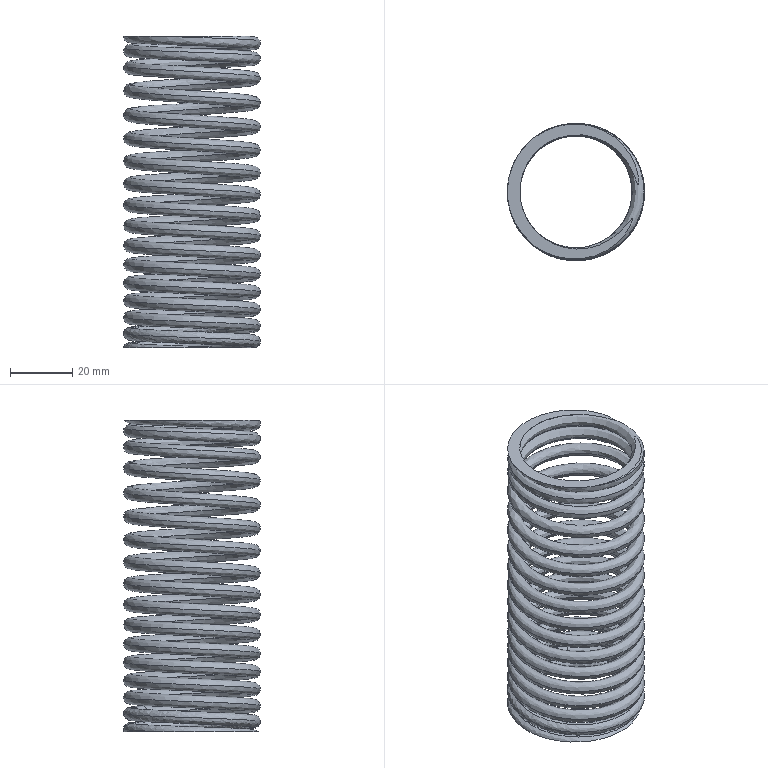Part | SolidWorks | features Helix 1, ICE 1, Sweep 1 | 1 solid | 7 faces | volume 25238 mm3 | spline 5 | plane 2